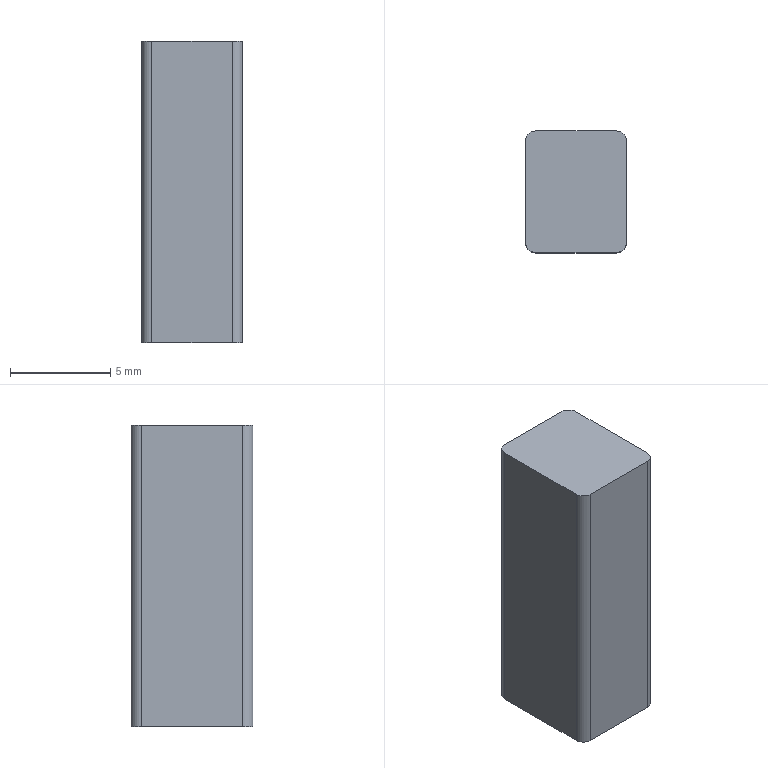Part | NX | features BREP 1 | 1 solid | 10 faces | box 5.03 x 6.05 x 15 mm | volume 453.248 mm3 | plane 6 | cylinder 4 | commonest cylinder face diameters 1 x4
STEP:
#1=CARTESIAN_POINT('',(-2.015,3.025,-25.6));
#2=VERTEX_POINT('',#1);
#3=CARTESIAN_POINT('',(-2.515,2.525,-25.6));
#4=VERTEX_POINT('',#3);
#5=CARTESIAN_POINT('',(-2.015,2.525,-25.6));
#6=DIRECTION('',(0.,0.,1.));
#7=DIRECTION('',(1.,0.,0.));
#8=AXIS2_PLACEMENT_3D('',#5,#6,#7);
#9=CIRCLE('',#8,0.5);
#10=EDGE_CURVE('',#2,#4,#9,.T.);
#11=ORIENTED_EDGE('',*,*,#10,.F.);
#12=CARTESIAN_POINT('',(-2.015,3.025,-40.6));
#13=VERTEX_POINT('',#12);
#14=CARTESIAN_POINT('',(-2.015,3.025,-40.6));
#15=DIRECTION('',(0.,0.,1.));
#16=VECTOR('',#15,1000.);
#17=LINE('',#14,#16);
#18=EDGE_CURVE('',#13,#2,#17,.T.);
#19=ORIENTED_EDGE('',*,*,#18,.F.);
#20=CARTESIAN_POINT('',(-2.515,2.525,-40.6));
#21=VERTEX_POINT('',#20);
#22=CARTESIAN_POINT('',(-2.015,2.525,-40.6));
#23=DIRECTION('',(0.,0.,1.));
#24=DIRECTION('',(1.,0.,0.));
#25=AXIS2_PLACEMENT_3D('',#22,#23,#24);
#26=CIRCLE('',#25,0.5);
#27=EDGE_CURVE('',#13,#21,#26,.T.);
#28=ORIENTED_EDGE('',*,*,#27,.T.);
#29=CARTESIAN_POINT('',(-2.515,2.525,-40.6));
#30=DIRECTION('',(0.,0.,1.));
#31=VECTOR('',#30,1000.);
#32=LINE('',#29,#31);
#33=EDGE_CURVE('',#21,#4,#32,.T.);
#34=ORIENTED_EDGE('',*,*,#33,.T.);
#35=EDGE_LOOP('',(#11,#19,#28,#34));
#36=FACE_BOUND('',#35,.T.);
#37=CARTESIAN_POINT('',(-2.015,2.525,-40.6));
#38=DIRECTION('',(0.,0.,1.));
#39=DIRECTION('',(-1.,0.,0.));
#40=AXIS2_PLACEMENT_3D('',#37,#38,#39);
#41=CYLINDRICAL_SURFACE('',#40,0.5);
#42=ADVANCED_FACE('',(#36),#41,.T.);
#43=CARTESIAN_POINT('',(-2.515,-2.525,-25.6));
#44=VERTEX_POINT('',#43);
#45=CARTESIAN_POINT('',(-2.515,-2.525,-25.6));
#46=DIRECTION('',(0.,1.,0.));
#47=VECTOR('',#46,1000.);
#48=LINE('',#45,#47);
#49=EDGE_CURVE('',#44,#4,#48,.T.);
#50=ORIENTED_EDGE('',*,*,#49,.T.);
#51=ORIENTED_EDGE('',*,*,#33,.F.);
#52=CARTESIAN_POINT('',(-2.515,-2.525,-40.6));
#53=VERTEX_POINT('',#52);
#54=CARTESIAN_POINT('',(-2.515,-2.525,-40.6));
#55=DIRECTION('',(0.,1.,0.));
#56=VECTOR('',#55,1000.);
#57=LINE('',#54,#56);
#58=EDGE_CURVE('',#53,#21,#57,.T.);
#59=ORIENTED_EDGE('',*,*,#58,.F.);
#60=CARTESIAN_POINT('',(-2.515,-2.525,-40.6));
#61=DIRECTION('',(0.,0.,1.));
#62=VECTOR('',#61,1000.);
#63=LINE('',#60,#62);
#64=EDGE_CURVE('',#53,#44,#63,.T.);
#65=ORIENTED_EDGE('',*,*,#64,.T.);
#66=EDGE_LOOP('',(#50,#51,#59,#65));
#67=FACE_BOUND('',#66,.T.);
#68=CARTESIAN_POINT('',(-2.515,-2.525,-40.6));
#69=DIRECTION('',(1.,0.,0.));
#70=DIRECTION('',(0.,0.,1.));
#71=AXIS2_PLACEMENT_3D('',#68,#69,#70);
#72=PLANE('',#71);
#73=ADVANCED_FACE('',(#67),#72,.F.);
#74=CARTESIAN_POINT('',(-2.015,-3.025,-25.6));
#75=VERTEX_POINT('',#74);
#76=CARTESIAN_POINT('',(-2.015,-2.525,-25.6));
#77=DIRECTION('',(0.,0.,1.));
#78=DIRECTION('',(1.,0.,0.));
#79=AXIS2_PLACEMENT_3D('',#76,#77,#78);
#80=CIRCLE('',#79,0.5);
#81=EDGE_CURVE('',#44,#75,#80,.T.);
#82=ORIENTED_EDGE('',*,*,#81,.F.);
#83=ORIENTED_EDGE('',*,*,#64,.F.);
#84=CARTESIAN_POINT('',(-2.015,-3.025,-40.6));
#85=VERTEX_POINT('',#84);
#86=CARTESIAN_POINT('',(-2.015,-2.525,-40.6));
#87=DIRECTION('',(0.,0.,1.));
#88=DIRECTION('',(1.,0.,0.));
#89=AXIS2_PLACEMENT_3D('',#86,#87,#88);
#90=CIRCLE('',#89,0.5);
#91=EDGE_CURVE('',#53,#85,#90,.T.);
#92=ORIENTED_EDGE('',*,*,#91,.T.);
#93=CARTESIAN_POINT('',(-2.015,-3.025,-40.6));
#94=DIRECTION('',(0.,0.,1.));
#95=VECTOR('',#94,1000.);
#96=LINE('',#93,#95);
#97=EDGE_CURVE('',#85,#75,#96,.T.);
#98=ORIENTED_EDGE('',*,*,#97,.T.);
#99=EDGE_LOOP('',(#82,#83,#92,#98));
#100=FACE_BOUND('',#99,.T.);
#101=CARTESIAN_POINT('',(-2.015,-2.525,-40.6));
#102=DIRECTION('',(0.,0.,1.));
#103=DIRECTION('',(-1.,0.,0.));
#104=AXIS2_PLACEMENT_3D('',#101,#102,#103);
#105=CYLINDRICAL_SURFACE('',#104,0.5);
#106=ADVANCED_FACE('',(#100),#105,.T.);
#107=CARTESIAN_POINT('',(2.015,-3.025,-25.6));
#108=VERTEX_POINT('',#107);
#109=CARTESIAN_POINT('',(2.015,-3.025,-25.6));
#110=DIRECTION('',(-1.,0.,0.));
#111=VECTOR('',#110,1000.);
#112=LINE('',#109,#111);
#113=EDGE_CURVE('',#108,#75,#112,.T.);
#114=ORIENTED_EDGE('',*,*,#113,.T.);
#115=ORIENTED_EDGE('',*,*,#97,.F.);
#116=CARTESIAN_POINT('',(2.015,-3.025,-40.6));
#117=VERTEX_POINT('',#116);
#118=CARTESIAN_POINT('',(2.015,-3.025,-40.6));
#119=DIRECTION('',(-1.,0.,0.));
#120=VECTOR('',#119,1000.);
#121=LINE('',#118,#120);
#122=EDGE_CURVE('',#117,#85,#121,.T.);
#123=ORIENTED_EDGE('',*,*,#122,.F.);
#124=CARTESIAN_POINT('',(2.015,-3.025,-40.6));
#125=DIRECTION('',(0.,0.,1.));
#126=VECTOR('',#125,1000.);
#127=LINE('',#124,#126);
#128=EDGE_CURVE('',#117,#108,#127,.T.);
#129=ORIENTED_EDGE('',*,*,#128,.T.);
#130=EDGE_LOOP('',(#114,#115,#123,#129));
#131=FACE_BOUND('',#130,.T.);
#132=CARTESIAN_POINT('',(2.015,-3.025,-40.6));
#133=DIRECTION('',(0.,1.,0.));
#134=DIRECTION('',(0.,0.,-1.));
#135=AXIS2_PLACEMENT_3D('',#132,#133,#134);
#136=PLANE('',#135);
#137=ADVANCED_FACE('',(#131),#136,.F.);
#138=CARTESIAN_POINT('',(2.515,-2.525,-25.6));
#139=VERTEX_POINT('',#138);
#140=CARTESIAN_POINT('',(2.015,-2.525,-25.6));
#141=DIRECTION('',(0.,0.,1.));
#142=DIRECTION('',(1.,0.,0.));
#143=AXIS2_PLACEMENT_3D('',#140,#141,#142);
#144=CIRCLE('',#143,0.5);
#145=EDGE_CURVE('',#108,#139,#144,.T.);
#146=ORIENTED_EDGE('',*,*,#145,.F.);
#147=ORIENTED_EDGE('',*,*,#128,.F.);
#148=CARTESIAN_POINT('',(2.515,-2.525,-40.6));
#149=VERTEX_POINT('',#148);
#150=CARTESIAN_POINT('',(2.015,-2.525,-40.6));
#151=DIRECTION('',(0.,0.,1.));
#152=DIRECTION('',(1.,0.,0.));
#153=AXIS2_PLACEMENT_3D('',#150,#151,#152);
#154=CIRCLE('',#153,0.5);
#155=EDGE_CURVE('',#117,#149,#154,.T.);
#156=ORIENTED_EDGE('',*,*,#155,.T.);
#157=CARTESIAN_POINT('',(2.515,-2.525,-40.6));
#158=DIRECTION('',(0.,0.,1.));
#159=VECTOR('',#158,1000.);
#160=LINE('',#157,#159);
#161=EDGE_CURVE('',#149,#139,#160,.T.);
#162=ORIENTED_EDGE('',*,*,#161,.T.);
#163=EDGE_LOOP('',(#146,#147,#156,#162));
#164=FACE_BOUND('',#163,.T.);
#165=CARTESIAN_POINT('',(2.015,-2.525,-40.6));
#166=DIRECTION('',(0.,0.,1.));
#167=DIRECTION('',(-1.,0.,0.));
#168=AXIS2_PLACEMENT_3D('',#165,#166,#167);
#169=CYLINDRICAL_SURFACE('',#168,0.5);
#170=ADVANCED_FACE('',(#164),#169,.T.);
#171=CARTESIAN_POINT('',(2.515,2.525,-25.6));
#172=VERTEX_POINT('',#171);
#173=CARTESIAN_POINT('',(2.515,2.525,-25.6));
#174=DIRECTION('',(0.,-1.,0.));
#175=VECTOR('',#174,1000.);
#176=LINE('',#173,#175);
#177=EDGE_CURVE('',#172,#139,#176,.T.);
#178=ORIENTED_EDGE('',*,*,#177,.T.);
#179=ORIENTED_EDGE('',*,*,#161,.F.);
#180=CARTESIAN_POINT('',(2.515,2.525,-40.6));
#181=VERTEX_POINT('',#180);
#182=CARTESIAN_POINT('',(2.515,2.525,-40.6));
#183=DIRECTION('',(0.,-1.,0.));
#184=VECTOR('',#183,1000.);
#185=LINE('',#182,#184);
#186=EDGE_CURVE('',#181,#149,#185,.T.);
#187=ORIENTED_EDGE('',*,*,#186,.F.);
#188=CARTESIAN_POINT('',(2.515,2.525,-40.6));
#189=DIRECTION('',(0.,0.,1.));
#190=VECTOR('',#189,1000.);
#191=LINE('',#188,#190);
#192=EDGE_CURVE('',#181,#172,#191,.T.);
#193=ORIENTED_EDGE('',*,*,#192,.T.);
#194=EDGE_LOOP('',(#178,#179,#187,#193));
#195=FACE_BOUND('',#194,.T.);
#196=CARTESIAN_POINT('',(2.515,2.525,-40.6));
#197=DIRECTION('',(-1.,0.,0.));
#198=DIRECTION('',(0.,0.,-1.));
#199=AXIS2_PLACEMENT_3D('',#196,#197,#198);
#200=PLANE('',#199);
#201=ADVANCED_FACE('',(#195),#200,.F.);
#202=CARTESIAN_POINT('',(2.015,3.025,-25.6));
#203=VERTEX_POINT('',#202);
#204=CARTESIAN_POINT('',(2.015,2.525,-25.6));
#205=DIRECTION('',(0.,0.,1.));
#206=DIRECTION('',(1.,0.,0.));
#207=AXIS2_PLACEMENT_3D('',#204,#205,#206);
#208=CIRCLE('',#207,0.5);
#209=EDGE_CURVE('',#172,#203,#208,.T.);
#210=ORIENTED_EDGE('',*,*,#209,.F.);
#211=ORIENTED_EDGE('',*,*,#192,.F.);
#212=CARTESIAN_POINT('',(2.015,3.025,-40.6));
#213=VERTEX_POINT('',#212);
#214=CARTESIAN_POINT('',(2.015,2.525,-40.6));
#215=DIRECTION('',(0.,0.,1.));
#216=DIRECTION('',(1.,0.,0.));
#217=AXIS2_PLACEMENT_3D('',#214,#215,#216);
#218=CIRCLE('',#217,0.5);
#219=EDGE_CURVE('',#181,#213,#218,.T.);
#220=ORIENTED_EDGE('',*,*,#219,.T.);
#221=CARTESIAN_POINT('',(2.015,3.025,-40.6));
#222=DIRECTION('',(0.,0.,1.));
#223=VECTOR('',#222,1000.);
#224=LINE('',#221,#223);
#225=EDGE_CURVE('',#213,#203,#224,.T.);
#226=ORIENTED_EDGE('',*,*,#225,.T.);
#227=EDGE_LOOP('',(#210,#211,#220,#226));
#228=FACE_BOUND('',#227,.T.);
#229=CARTESIAN_POINT('',(2.015,2.525,-40.6));
#230=DIRECTION('',(0.,0.,1.));
#231=DIRECTION('',(-1.,0.,0.));
#232=AXIS2_PLACEMENT_3D('',#229,#230,#231);
#233=CYLINDRICAL_SURFACE('',#232,0.5);
#234=ADVANCED_FACE('',(#228),#233,.T.);
#235=CARTESIAN_POINT('',(-2.015,3.025,-25.6));
#236=DIRECTION('',(1.,0.,0.));
#237=VECTOR('',#236,1000.);
#238=LINE('',#235,#237);
#239=EDGE_CURVE('',#2,#203,#238,.T.);
#240=ORIENTED_EDGE('',*,*,#239,.T.);
#241=ORIENTED_EDGE('',*,*,#225,.F.);
#242=CARTESIAN_POINT('',(-2.015,3.025,-40.6));
#243=DIRECTION('',(1.,0.,0.));
#244=VECTOR('',#243,1000.);
#245=LINE('',#242,#244);
#246=EDGE_CURVE('',#13,#213,#245,.T.);
#247=ORIENTED_EDGE('',*,*,#246,.F.);
#248=ORIENTED_EDGE('',*,*,#18,.T.);
#249=EDGE_LOOP('',(#240,#241,#247,#248));
#250=FACE_BOUND('',#249,.T.);
#251=CARTESIAN_POINT('',(-2.015,3.025,-40.6));
#252=DIRECTION('',(0.,-1.,0.));
#253=DIRECTION('',(0.,0.,1.));
#254=AXIS2_PLACEMENT_3D('',#251,#252,#253);
#255=PLANE('',#254);
#256=ADVANCED_FACE('',(#250),#255,.F.);
#257=ORIENTED_EDGE('',*,*,#27,.F.);
#258=ORIENTED_EDGE('',*,*,#246,.T.);
#259=ORIENTED_EDGE('',*,*,#219,.F.);
#260=ORIENTED_EDGE('',*,*,#186,.T.);
#261=ORIENTED_EDGE('',*,*,#155,.F.);
#262=ORIENTED_EDGE('',*,*,#122,.T.);
#263=ORIENTED_EDGE('',*,*,#91,.F.);
#264=ORIENTED_EDGE('',*,*,#58,.T.);
#265=EDGE_LOOP('',(#257,#258,#259,#260,#261,#262,#263,#264));
#266=FACE_BOUND('',#265,.T.);
#267=CARTESIAN_POINT('',(-2.015,2.525,-40.6));
#268=DIRECTION('',(0.,0.,1.));
#269=DIRECTION('',(-1.,0.,0.));
#270=AXIS2_PLACEMENT_3D('',#267,#268,#269);
#271=PLANE('',#270);
#272=ADVANCED_FACE('',(#266),#271,.F.);
#273=ORIENTED_EDGE('',*,*,#10,.T.);
#274=ORIENTED_EDGE('',*,*,#49,.F.);
#275=ORIENTED_EDGE('',*,*,#81,.T.);
#276=ORIENTED_EDGE('',*,*,#113,.F.);
#277=ORIENTED_EDGE('',*,*,#145,.T.);
#278=ORIENTED_EDGE('',*,*,#177,.F.);
#279=ORIENTED_EDGE('',*,*,#209,.T.);
#280=ORIENTED_EDGE('',*,*,#239,.F.);
#281=EDGE_LOOP('',(#273,#274,#275,#276,#277,#278,#279,#280));
#282=FACE_BOUND('',#281,.T.);
#283=CARTESIAN_POINT('',(-2.015,2.525,-25.6));
#284=DIRECTION('',(0.,0.,1.));
#285=DIRECTION('',(-1.,0.,0.));
#286=AXIS2_PLACEMENT_3D('',#283,#284,#285);
#287=PLANE('',#286);
#288=ADVANCED_FACE('',(#282),#287,.T.);
#289=CLOSED_SHELL('',(#42,#73,#106,#137,#170,#201,#234,#256,#272,#288));
#290=MANIFOLD_SOLID_BREP('',#289);
#291=(LENGTH_UNIT()NAMED_UNIT(*)SI_UNIT(.MILLI.,.METRE.));
#292=UNCERTAINTY_MEASURE_WITH_UNIT(LENGTH_MEASURE(0.00001),#291,'','');
#293=(NAMED_UNIT(*)PLANE_ANGLE_UNIT()SI_UNIT($,.RADIAN.));
#294=(NAMED_UNIT(*)SI_UNIT($,.STERADIAN.)SOLID_ANGLE_UNIT());
#295=(GEOMETRIC_REPRESENTATION_CONTEXT(3)GLOBAL_UNCERTAINTY_ASSIGNED_CONTEXT((#292))GLOBAL_UNIT_ASSIGNED_CONTEXT((#291,#293,#294))REPRESENTATION_CONTEXT('',''));
#296=ADVANCED_BREP_SHAPE_REPRESENTATION('',(#290),#295);